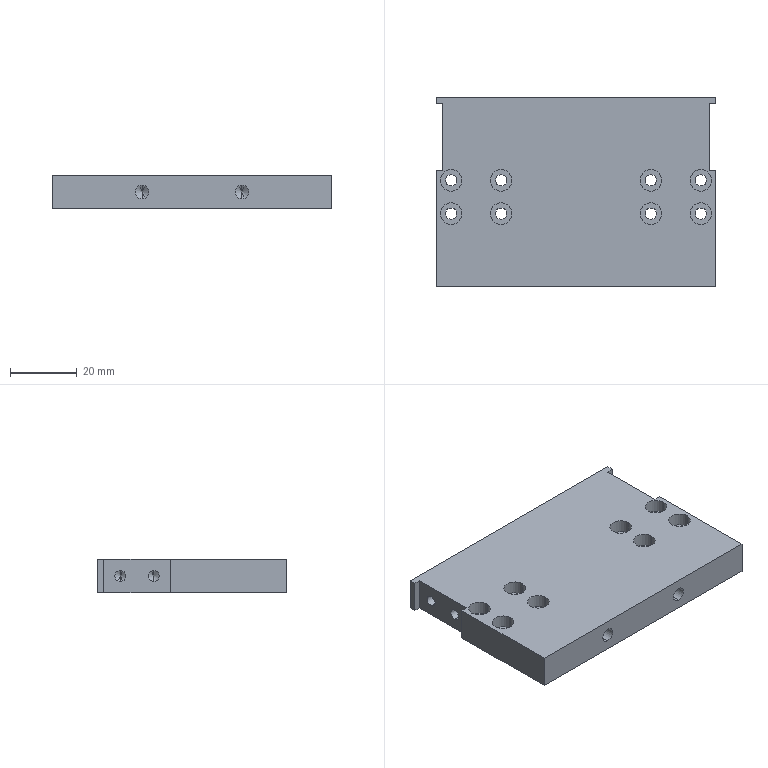Part | STEP file | 227H056248 JIG Block | 1 solid | 86 faces | box 84 x 57 x 10 mm | volume 44690 mm3 | cylinder 48 | plane 22 | cone 16 | commonest cylinder face diameters 3.4 x16 6.5 x16 3.3 x12 4.2 x4